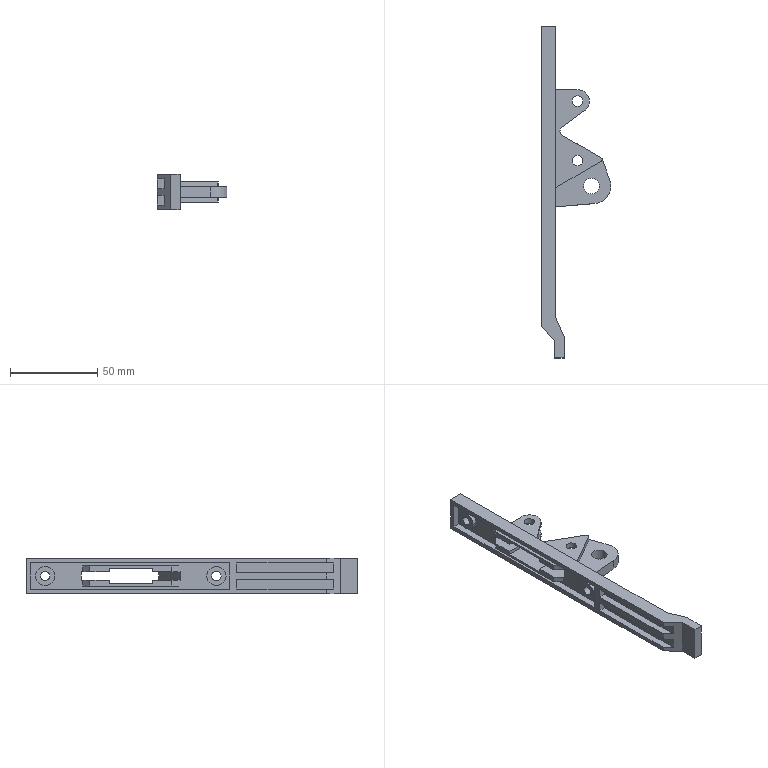Part | STEP file | 1 solid | 92 faces | box 39.772 x 190 x 20.1 mm | volume 27752 mm3 | plane 60 | cylinder 28 | cone 4 | commonest cylinder face diameters 6 x10 5.3 x4 11 x4 13 x4 2 x3 9 x2